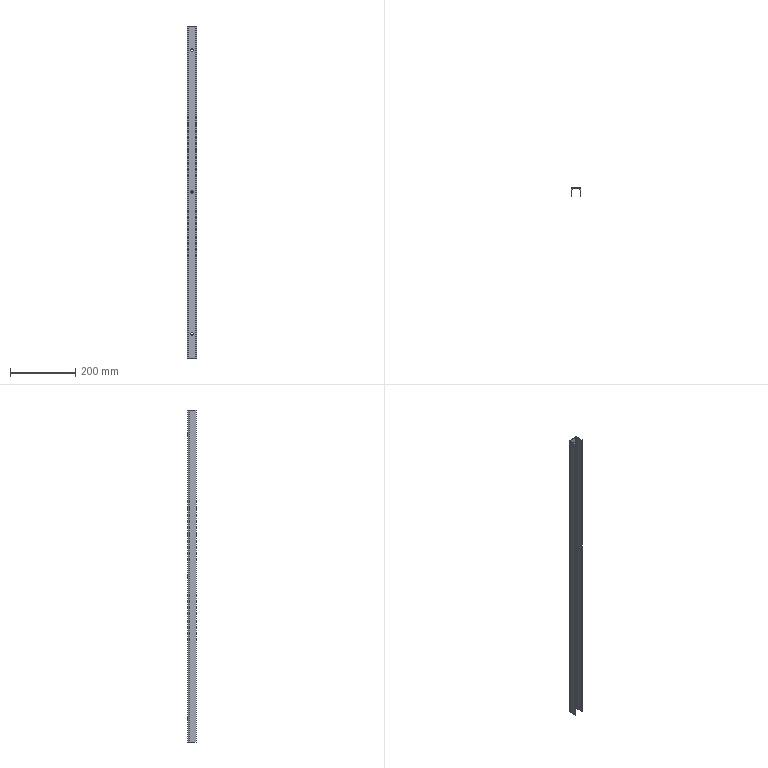Part | STEP file | SYL_0392D6J1SYL0380DJ10-1470572 | 1 solid | 28 faces | box 30 x 25 x 1018 mm | volume 149191 mm3 | plane 18 | cylinder 10 | commonest cylinder face diameters 8 x8 4 x2
STEP:
#1=CARTESIAN_POINT('',(0.,23.,-439.));
#2=VERTEX_POINT('',#1);
#3=CARTESIAN_POINT('',(0.,25.,-439.));
#4=VERTEX_POINT('',#3);
#5=CARTESIAN_POINT('',(0.,25.,-439.));
#6=DIRECTION('',(0.,1.,0.));
#7=VECTOR('',#6,1000.);
#8=LINE('',#5,#7);
#9=EDGE_CURVE('',#2,#4,#8,.T.);
#10=ORIENTED_EDGE('',*,*,#9,.F.);
#11=CARTESIAN_POINT('',(0.,23.,-431.));
#12=VERTEX_POINT('',#11);
#13=CARTESIAN_POINT('',(0.,23.,-435.));
#14=DIRECTION('',(0.,-1.,0.));
#15=DIRECTION('',(0.,0.,-1.));
#16=AXIS2_PLACEMENT_3D('',#13,#14,#15);
#17=CIRCLE('',#16,4.);
#18=EDGE_CURVE('',#2,#12,#17,.T.);
#19=ORIENTED_EDGE('',*,*,#18,.T.);
#20=CARTESIAN_POINT('',(0.,25.,-431.));
#21=VERTEX_POINT('',#20);
#22=CARTESIAN_POINT('',(0.,25.,-431.));
#23=DIRECTION('',(0.,1.,0.));
#24=VECTOR('',#23,1000.);
#25=LINE('',#22,#24);
#26=EDGE_CURVE('',#12,#21,#25,.T.);
#27=ORIENTED_EDGE('',*,*,#26,.T.);
#28=CARTESIAN_POINT('',(0.,25.,-435.));
#29=DIRECTION('',(0.,-1.,0.));
#30=DIRECTION('',(0.,0.,-1.));
#31=AXIS2_PLACEMENT_3D('',#28,#29,#30);
#32=CIRCLE('',#31,4.);
#33=EDGE_CURVE('',#4,#21,#32,.T.);
#34=ORIENTED_EDGE('',*,*,#33,.F.);
#35=EDGE_LOOP('',(#10,#19,#27,#34));
#36=FACE_OUTER_BOUND('',#35,.T.);
#37=CARTESIAN_POINT('',(0.,25.,-435.));
#38=DIRECTION('',(0.,1.,0.));
#39=DIRECTION('',(0.,0.,1.));
#40=AXIS2_PLACEMENT_3D('',#37,#38,#39);
#41=CYLINDRICAL_SURFACE('',#40,4.);
#42=ADVANCED_FACE('',(#36),#41,.F.);
#43=CARTESIAN_POINT('',(0.,23.,-4.));
#44=VERTEX_POINT('',#43);
#45=CARTESIAN_POINT('',(0.,25.,-4.));
#46=VERTEX_POINT('',#45);
#47=CARTESIAN_POINT('',(0.,25.,-4.));
#48=DIRECTION('',(0.,1.,0.));
#49=VECTOR('',#48,1000.);
#50=LINE('',#47,#49);
#51=EDGE_CURVE('',#44,#46,#50,.T.);
#52=ORIENTED_EDGE('',*,*,#51,.F.);
#53=CARTESIAN_POINT('',(0.,23.,4.));
#54=VERTEX_POINT('',#53);
#55=CARTESIAN_POINT('',(0.,23.,0.));
#56=DIRECTION('',(0.,-1.,0.));
#57=DIRECTION('',(0.,0.,-1.));
#58=AXIS2_PLACEMENT_3D('',#55,#56,#57);
#59=CIRCLE('',#58,4.);
#60=EDGE_CURVE('',#44,#54,#59,.T.);
#61=ORIENTED_EDGE('',*,*,#60,.T.);
#62=CARTESIAN_POINT('',(0.,25.,4.));
#63=VERTEX_POINT('',#62);
#64=CARTESIAN_POINT('',(0.,25.,4.));
#65=DIRECTION('',(0.,1.,0.));
#66=VECTOR('',#65,1000.);
#67=LINE('',#64,#66);
#68=EDGE_CURVE('',#54,#63,#67,.T.);
#69=ORIENTED_EDGE('',*,*,#68,.T.);
#70=CARTESIAN_POINT('',(0.,25.,0.));
#71=DIRECTION('',(0.,-1.,0.));
#72=DIRECTION('',(0.,0.,-1.));
#73=AXIS2_PLACEMENT_3D('',#70,#71,#72);
#74=CIRCLE('',#73,4.);
#75=EDGE_CURVE('',#46,#63,#74,.T.);
#76=ORIENTED_EDGE('',*,*,#75,.F.);
#77=EDGE_LOOP('',(#52,#61,#69,#76));
#78=FACE_OUTER_BOUND('',#77,.T.);
#79=CARTESIAN_POINT('',(0.,25.,0.));
#80=DIRECTION('',(0.,1.,0.));
#81=DIRECTION('',(0.,0.,1.));
#82=AXIS2_PLACEMENT_3D('',#79,#80,#81);
#83=CYLINDRICAL_SURFACE('',#82,4.);
#84=ADVANCED_FACE('',(#78),#83,.F.);
#85=CARTESIAN_POINT('',(0.,23.,431.));
#86=VERTEX_POINT('',#85);
#87=CARTESIAN_POINT('',(0.,25.,431.));
#88=VERTEX_POINT('',#87);
#89=CARTESIAN_POINT('',(0.,25.,431.));
#90=DIRECTION('',(0.,1.,0.));
#91=VECTOR('',#90,1000.);
#92=LINE('',#89,#91);
#93=EDGE_CURVE('',#86,#88,#92,.T.);
#94=ORIENTED_EDGE('',*,*,#93,.F.);
#95=CARTESIAN_POINT('',(0.,23.,439.));
#96=VERTEX_POINT('',#95);
#97=CARTESIAN_POINT('',(0.,23.,435.));
#98=DIRECTION('',(0.,-1.,0.));
#99=DIRECTION('',(0.,0.,-1.));
#100=AXIS2_PLACEMENT_3D('',#97,#98,#99);
#101=CIRCLE('',#100,4.);
#102=EDGE_CURVE('',#86,#96,#101,.T.);
#103=ORIENTED_EDGE('',*,*,#102,.T.);
#104=CARTESIAN_POINT('',(0.,25.,439.));
#105=VERTEX_POINT('',#104);
#106=CARTESIAN_POINT('',(0.,25.,439.));
#107=DIRECTION('',(0.,1.,0.));
#108=VECTOR('',#107,1000.);
#109=LINE('',#106,#108);
#110=EDGE_CURVE('',#96,#105,#109,.T.);
#111=ORIENTED_EDGE('',*,*,#110,.T.);
#112=CARTESIAN_POINT('',(0.,25.,435.));
#113=DIRECTION('',(0.,-1.,0.));
#114=DIRECTION('',(0.,0.,-1.));
#115=AXIS2_PLACEMENT_3D('',#112,#113,#114);
#116=CIRCLE('',#115,4.);
#117=EDGE_CURVE('',#88,#105,#116,.T.);
#118=ORIENTED_EDGE('',*,*,#117,.F.);
#119=EDGE_LOOP('',(#94,#103,#111,#118));
#120=FACE_OUTER_BOUND('',#119,.T.);
#121=CARTESIAN_POINT('',(0.,25.,435.));
#122=DIRECTION('',(0.,1.,0.));
#123=DIRECTION('',(0.,0.,1.));
#124=AXIS2_PLACEMENT_3D('',#121,#122,#123);
#125=CYLINDRICAL_SURFACE('',#124,4.);
#126=ADVANCED_FACE('',(#120),#125,.F.);
#127=CARTESIAN_POINT('',(-13.,0.,-509.));
#128=VERTEX_POINT('',#127);
#129=CARTESIAN_POINT('',(-15.,0.,-509.));
#130=VERTEX_POINT('',#129);
#131=CARTESIAN_POINT('',(-15.,0.,-509.));
#132=DIRECTION('',(-1.,0.,0.));
#133=VECTOR('',#132,1000.);
#134=LINE('',#131,#133);
#135=EDGE_CURVE('',#128,#130,#134,.T.);
#136=ORIENTED_EDGE('',*,*,#135,.F.);
#137=CARTESIAN_POINT('',(-13.,0.,509.));
#138=VERTEX_POINT('',#137);
#139=CARTESIAN_POINT('',(-13.,0.,-509.));
#140=DIRECTION('',(0.,0.,1.));
#141=VECTOR('',#140,1000.);
#142=LINE('',#139,#141);
#143=EDGE_CURVE('',#128,#138,#142,.T.);
#144=ORIENTED_EDGE('',*,*,#143,.T.);
#145=CARTESIAN_POINT('',(-15.,0.,509.));
#146=VERTEX_POINT('',#145);
#147=CARTESIAN_POINT('',(-15.,0.,509.));
#148=DIRECTION('',(-1.,0.,0.));
#149=VECTOR('',#148,1000.);
#150=LINE('',#147,#149);
#151=EDGE_CURVE('',#138,#146,#150,.T.);
#152=ORIENTED_EDGE('',*,*,#151,.T.);
#153=CARTESIAN_POINT('',(-15.,0.,-509.));
#154=DIRECTION('',(0.,0.,1.));
#155=VECTOR('',#154,1000.);
#156=LINE('',#153,#155);
#157=EDGE_CURVE('',#130,#146,#156,.T.);
#158=ORIENTED_EDGE('',*,*,#157,.F.);
#159=EDGE_LOOP('',(#136,#144,#152,#158));
#160=FACE_OUTER_BOUND('',#159,.T.);
#161=CARTESIAN_POINT('',(-15.,0.,-509.));
#162=DIRECTION('',(0.,-1.,0.));
#163=DIRECTION('',(0.,0.,1.));
#164=AXIS2_PLACEMENT_3D('',#161,#162,#163);
#165=PLANE('',#164);
#166=ADVANCED_FACE('',(#160),#165,.T.);
#167=ORIENTED_EDGE('',*,*,#151,.F.);
#168=CARTESIAN_POINT('',(-13.,21.,509.));
#169=VERTEX_POINT('',#168);
#170=CARTESIAN_POINT('',(-13.,21.,509.));
#171=DIRECTION('',(0.,-1.,0.));
#172=VECTOR('',#171,1000.);
#173=LINE('',#170,#172);
#174=EDGE_CURVE('',#169,#138,#173,.T.);
#175=ORIENTED_EDGE('',*,*,#174,.F.);
#176=CARTESIAN_POINT('',(-15.,21.,509.));
#177=VERTEX_POINT('',#176);
#178=CARTESIAN_POINT('',(-15.,21.,509.));
#179=DIRECTION('',(-1.,0.,0.));
#180=VECTOR('',#179,1000.);
#181=LINE('',#178,#180);
#182=EDGE_CURVE('',#169,#177,#181,.T.);
#183=ORIENTED_EDGE('',*,*,#182,.T.);
#184=CARTESIAN_POINT('',(-15.,21.,509.));
#185=DIRECTION('',(0.,-1.,0.));
#186=VECTOR('',#185,1000.);
#187=LINE('',#184,#186);
#188=EDGE_CURVE('',#177,#146,#187,.T.);
#189=ORIENTED_EDGE('',*,*,#188,.T.);
#190=EDGE_LOOP('',(#167,#175,#183,#189));
#191=FACE_OUTER_BOUND('',#190,.T.);
#192=CARTESIAN_POINT('',(-15.,21.,509.));
#193=DIRECTION('',(0.,0.,-1.));
#194=DIRECTION('',(0.,-1.,0.));
#195=AXIS2_PLACEMENT_3D('',#192,#193,#194);
#196=PLANE('',#195);
#197=ADVANCED_FACE('',(#191),#196,.F.);
#198=ORIENTED_EDGE('',*,*,#182,.F.);
#199=CARTESIAN_POINT('',(-11.,23.,509.));
#200=VERTEX_POINT('',#199);
#201=CARTESIAN_POINT('',(-11.,21.,509.));
#202=DIRECTION('',(0.,0.,1.));
#203=DIRECTION('',(1.,0.,0.));
#204=AXIS2_PLACEMENT_3D('',#201,#202,#203);
#205=CIRCLE('',#204,2.);
#206=EDGE_CURVE('',#200,#169,#205,.T.);
#207=ORIENTED_EDGE('',*,*,#206,.F.);
#208=CARTESIAN_POINT('',(-11.,25.,509.));
#209=VERTEX_POINT('',#208);
#210=CARTESIAN_POINT('',(-11.,25.,509.));
#211=DIRECTION('',(0.,1.,0.));
#212=VECTOR('',#211,1000.);
#213=LINE('',#210,#212);
#214=EDGE_CURVE('',#200,#209,#213,.T.);
#215=ORIENTED_EDGE('',*,*,#214,.T.);
#216=CARTESIAN_POINT('',(-11.,21.,509.));
#217=DIRECTION('',(0.,0.,1.));
#218=DIRECTION('',(0.,1.,0.));
#219=AXIS2_PLACEMENT_3D('',#216,#217,#218);
#220=CIRCLE('',#219,4.);
#221=EDGE_CURVE('',#209,#177,#220,.T.);
#222=ORIENTED_EDGE('',*,*,#221,.T.);
#223=EDGE_LOOP('',(#198,#207,#215,#222));
#224=FACE_OUTER_BOUND('',#223,.T.);
#225=CARTESIAN_POINT('',(-11.,21.,509.));
#226=DIRECTION('',(0.,0.,-1.));
#227=DIRECTION('',(-1.,0.,0.));
#228=AXIS2_PLACEMENT_3D('',#225,#226,#227);
#229=PLANE('',#228);
#230=ADVANCED_FACE('',(#224),#229,.F.);
#231=ORIENTED_EDGE('',*,*,#214,.F.);
#232=CARTESIAN_POINT('',(11.,23.,509.));
#233=VERTEX_POINT('',#232);
#234=CARTESIAN_POINT('',(11.,23.,509.));
#235=DIRECTION('',(-1.,0.,0.));
#236=VECTOR('',#235,1000.);
#237=LINE('',#234,#236);
#238=EDGE_CURVE('',#233,#200,#237,.T.);
#239=ORIENTED_EDGE('',*,*,#238,.F.);
#240=CARTESIAN_POINT('',(11.,25.,509.));
#241=VERTEX_POINT('',#240);
#242=CARTESIAN_POINT('',(11.,25.,509.));
#243=DIRECTION('',(0.,1.,0.));
#244=VECTOR('',#243,1000.);
#245=LINE('',#242,#244);
#246=EDGE_CURVE('',#233,#241,#245,.T.);
#247=ORIENTED_EDGE('',*,*,#246,.T.);
#248=CARTESIAN_POINT('',(11.,25.,509.));
#249=DIRECTION('',(-1.,0.,0.));
#250=VECTOR('',#249,1000.);
#251=LINE('',#248,#250);
#252=EDGE_CURVE('',#241,#209,#251,.T.);
#253=ORIENTED_EDGE('',*,*,#252,.T.);
#254=EDGE_LOOP('',(#231,#239,#247,#253));
#255=FACE_OUTER_BOUND('',#254,.T.);
#256=CARTESIAN_POINT('',(11.,25.,509.));
#257=DIRECTION('',(0.,0.,-1.));
#258=DIRECTION('',(-1.,0.,0.));
#259=AXIS2_PLACEMENT_3D('',#256,#257,#258);
#260=PLANE('',#259);
#261=ADVANCED_FACE('',(#255),#260,.F.);
#262=ORIENTED_EDGE('',*,*,#246,.F.);
#263=CARTESIAN_POINT('',(13.,21.,509.));
#264=VERTEX_POINT('',#263);
#265=CARTESIAN_POINT('',(11.,21.,509.));
#266=DIRECTION('',(0.,0.,1.));
#267=DIRECTION('',(1.,0.,0.));
#268=AXIS2_PLACEMENT_3D('',#265,#266,#267);
#269=CIRCLE('',#268,2.);
#270=EDGE_CURVE('',#264,#233,#269,.T.);
#271=ORIENTED_EDGE('',*,*,#270,.F.);
#272=CARTESIAN_POINT('',(15.,21.,509.));
#273=VERTEX_POINT('',#272);
#274=CARTESIAN_POINT('',(15.,21.,509.));
#275=DIRECTION('',(1.,0.,0.));
#276=VECTOR('',#275,1000.);
#277=LINE('',#274,#276);
#278=EDGE_CURVE('',#264,#273,#277,.T.);
#279=ORIENTED_EDGE('',*,*,#278,.T.);
#280=CARTESIAN_POINT('',(11.,21.,509.));
#281=DIRECTION('',(0.,0.,1.));
#282=DIRECTION('',(1.,0.,0.));
#283=AXIS2_PLACEMENT_3D('',#280,#281,#282);
#284=CIRCLE('',#283,4.);
#285=EDGE_CURVE('',#273,#241,#284,.T.);
#286=ORIENTED_EDGE('',*,*,#285,.T.);
#287=EDGE_LOOP('',(#262,#271,#279,#286));
#288=FACE_OUTER_BOUND('',#287,.T.);
#289=CARTESIAN_POINT('',(11.,21.,509.));
#290=DIRECTION('',(0.,0.,-1.));
#291=DIRECTION('',(-1.,0.,0.));
#292=AXIS2_PLACEMENT_3D('',#289,#290,#291);
#293=PLANE('',#292);
#294=ADVANCED_FACE('',(#288),#293,.F.);
#295=ORIENTED_EDGE('',*,*,#278,.F.);
#296=CARTESIAN_POINT('',(13.,0.,509.));
#297=VERTEX_POINT('',#296);
#298=CARTESIAN_POINT('',(13.,0.,509.));
#299=DIRECTION('',(0.,1.,0.));
#300=VECTOR('',#299,1000.);
#301=LINE('',#298,#300);
#302=EDGE_CURVE('',#297,#264,#301,.T.);
#303=ORIENTED_EDGE('',*,*,#302,.F.);
#304=CARTESIAN_POINT('',(15.,0.,509.));
#305=VERTEX_POINT('',#304);
#306=CARTESIAN_POINT('',(15.,0.,509.));
#307=DIRECTION('',(1.,0.,0.));
#308=VECTOR('',#307,1000.);
#309=LINE('',#306,#308);
#310=EDGE_CURVE('',#297,#305,#309,.T.);
#311=ORIENTED_EDGE('',*,*,#310,.T.);
#312=CARTESIAN_POINT('',(15.,0.,509.));
#313=DIRECTION('',(0.,1.,0.));
#314=VECTOR('',#313,1000.);
#315=LINE('',#312,#314);
#316=EDGE_CURVE('',#305,#273,#315,.T.);
#317=ORIENTED_EDGE('',*,*,#316,.T.);
#318=EDGE_LOOP('',(#295,#303,#311,#317));
#319=FACE_OUTER_BOUND('',#318,.T.);
#320=CARTESIAN_POINT('',(15.,0.,509.));
#321=DIRECTION('',(0.,0.,-1.));
#322=DIRECTION('',(0.,1.,0.));
#323=AXIS2_PLACEMENT_3D('',#320,#321,#322);
#324=PLANE('',#323);
#325=ADVANCED_FACE('',(#319),#324,.F.);
#326=ORIENTED_EDGE('',*,*,#310,.F.);
#327=CARTESIAN_POINT('',(13.,0.,-509.));
#328=VERTEX_POINT('',#327);
#329=CARTESIAN_POINT('',(13.,0.,-509.));
#330=DIRECTION('',(0.,0.,1.));
#331=VECTOR('',#330,1000.);
#332=LINE('',#329,#331);
#333=EDGE_CURVE('',#328,#297,#332,.T.);
#334=ORIENTED_EDGE('',*,*,#333,.F.);
#335=CARTESIAN_POINT('',(15.,0.,-509.));
#336=VERTEX_POINT('',#335);
#337=CARTESIAN_POINT('',(15.,0.,-509.));
#338=DIRECTION('',(1.,0.,0.));
#339=VECTOR('',#338,1000.);
#340=LINE('',#337,#339);
#341=EDGE_CURVE('',#328,#336,#340,.T.);
#342=ORIENTED_EDGE('',*,*,#341,.T.);
#343=CARTESIAN_POINT('',(15.,0.,-509.));
#344=DIRECTION('',(0.,0.,1.));
#345=VECTOR('',#344,1000.);
#346=LINE('',#343,#345);
#347=EDGE_CURVE('',#336,#305,#346,.T.);
#348=ORIENTED_EDGE('',*,*,#347,.T.);
#349=EDGE_LOOP('',(#326,#334,#342,#348));
#350=FACE_OUTER_BOUND('',#349,.T.);
#351=CARTESIAN_POINT('',(15.,0.,-509.));
#352=DIRECTION('',(0.,1.,0.));
#353=DIRECTION('',(0.,0.,1.));
#354=AXIS2_PLACEMENT_3D('',#351,#352,#353);
#355=PLANE('',#354);
#356=ADVANCED_FACE('',(#350),#355,.F.);
#357=ORIENTED_EDGE('',*,*,#341,.F.);
#358=CARTESIAN_POINT('',(13.,21.,-509.));
#359=VERTEX_POINT('',#358);
#360=CARTESIAN_POINT('',(13.,0.,-509.));
#361=DIRECTION('',(0.,1.,0.));
#362=VECTOR('',#361,1000.);
#363=LINE('',#360,#362);
#364=EDGE_CURVE('',#328,#359,#363,.T.);
#365=ORIENTED_EDGE('',*,*,#364,.T.);
#366=CARTESIAN_POINT('',(15.,21.,-509.));
#367=VERTEX_POINT('',#366);
#368=CARTESIAN_POINT('',(15.,21.,-509.));
#369=DIRECTION('',(1.,0.,0.));
#370=VECTOR('',#369,1000.);
#371=LINE('',#368,#370);
#372=EDGE_CURVE('',#359,#367,#371,.T.);
#373=ORIENTED_EDGE('',*,*,#372,.T.);
#374=CARTESIAN_POINT('',(15.,0.,-509.));
#375=DIRECTION('',(0.,1.,0.));
#376=VECTOR('',#375,1000.);
#377=LINE('',#374,#376);
#378=EDGE_CURVE('',#336,#367,#377,.T.);
#379=ORIENTED_EDGE('',*,*,#378,.F.);
#380=EDGE_LOOP('',(#357,#365,#373,#379));
#381=FACE_OUTER_BOUND('',#380,.T.);
#382=CARTESIAN_POINT('',(15.,0.,-509.));
#383=DIRECTION('',(0.,0.,-1.));
#384=DIRECTION('',(0.,1.,0.));
#385=AXIS2_PLACEMENT_3D('',#382,#383,#384);
#386=PLANE('',#385);
#387=ADVANCED_FACE('',(#381),#386,.T.);
#388=ORIENTED_EDGE('',*,*,#372,.F.);
#389=CARTESIAN_POINT('',(11.,23.,-509.));
#390=VERTEX_POINT('',#389);
#391=CARTESIAN_POINT('',(11.,21.,-509.));
#392=DIRECTION('',(0.,0.,-1.));
#393=DIRECTION('',(1.,0.,0.));
#394=AXIS2_PLACEMENT_3D('',#391,#392,#393);
#395=CIRCLE('',#394,2.);
#396=EDGE_CURVE('',#390,#359,#395,.T.);
#397=ORIENTED_EDGE('',*,*,#396,.F.);
#398=CARTESIAN_POINT('',(11.,25.,-509.));
#399=VERTEX_POINT('',#398);
#400=CARTESIAN_POINT('',(11.,25.,-509.));
#401=DIRECTION('',(0.,1.,0.));
#402=VECTOR('',#401,1000.);
#403=LINE('',#400,#402);
#404=EDGE_CURVE('',#390,#399,#403,.T.);
#405=ORIENTED_EDGE('',*,*,#404,.T.);
#406=CARTESIAN_POINT('',(11.,21.,-509.));
#407=DIRECTION('',(0.,0.,-1.));
#408=DIRECTION('',(0.,1.,0.));
#409=AXIS2_PLACEMENT_3D('',#406,#407,#408);
#410=CIRCLE('',#409,4.);
#411=EDGE_CURVE('',#399,#367,#410,.T.);
#412=ORIENTED_EDGE('',*,*,#411,.T.);
#413=EDGE_LOOP('',(#388,#397,#405,#412));
#414=FACE_OUTER_BOUND('',#413,.T.);
#415=CARTESIAN_POINT('',(11.,21.,-509.));
#416=DIRECTION('',(0.,0.,1.));
#417=DIRECTION('',(1.,0.,0.));
#418=AXIS2_PLACEMENT_3D('',#415,#416,#417);
#419=PLANE('',#418);
#420=ADVANCED_FACE('',(#414),#419,.F.);
#421=ORIENTED_EDGE('',*,*,#404,.F.);
#422=CARTESIAN_POINT('',(-11.,23.,-509.));
#423=VERTEX_POINT('',#422);
#424=CARTESIAN_POINT('',(11.,23.,-509.));
#425=DIRECTION('',(-1.,0.,0.));
#426=VECTOR('',#425,1000.);
#427=LINE('',#424,#426);
#428=EDGE_CURVE('',#390,#423,#427,.T.);
#429=ORIENTED_EDGE('',*,*,#428,.T.);
#430=CARTESIAN_POINT('',(-11.,25.,-509.));
#431=VERTEX_POINT('',#430);
#432=CARTESIAN_POINT('',(-11.,25.,-509.));
#433=DIRECTION('',(0.,1.,0.));
#434=VECTOR('',#433,1000.);
#435=LINE('',#432,#434);
#436=EDGE_CURVE('',#423,#431,#435,.T.);
#437=ORIENTED_EDGE('',*,*,#436,.T.);
#438=CARTESIAN_POINT('',(11.,25.,-509.));
#439=DIRECTION('',(-1.,0.,0.));
#440=VECTOR('',#439,1000.);
#441=LINE('',#438,#440);
#442=EDGE_CURVE('',#399,#431,#441,.T.);
#443=ORIENTED_EDGE('',*,*,#442,.F.);
#444=EDGE_LOOP('',(#421,#429,#437,#443));
#445=FACE_OUTER_BOUND('',#444,.T.);
#446=CARTESIAN_POINT('',(11.,25.,-509.));
#447=DIRECTION('',(0.,0.,-1.));
#448=DIRECTION('',(-1.,0.,0.));
#449=AXIS2_PLACEMENT_3D('',#446,#447,#448);
#450=PLANE('',#449);
#451=ADVANCED_FACE('',(#445),#450,.T.);
#452=ORIENTED_EDGE('',*,*,#436,.F.);
#453=CARTESIAN_POINT('',(-13.,21.,-509.));
#454=VERTEX_POINT('',#453);
#455=CARTESIAN_POINT('',(-11.,21.,-509.));
#456=DIRECTION('',(0.,0.,-1.));
#457=DIRECTION('',(1.,0.,0.));
#458=AXIS2_PLACEMENT_3D('',#455,#456,#457);
#459=CIRCLE('',#458,2.);
#460=EDGE_CURVE('',#454,#423,#459,.T.);
#461=ORIENTED_EDGE('',*,*,#460,.F.);
#462=CARTESIAN_POINT('',(-15.,21.,-509.));
#463=VERTEX_POINT('',#462);
#464=CARTESIAN_POINT('',(-15.,21.,-509.));
#465=DIRECTION('',(-1.,0.,0.));
#466=VECTOR('',#465,1000.);
#467=LINE('',#464,#466);
#468=EDGE_CURVE('',#454,#463,#467,.T.);
#469=ORIENTED_EDGE('',*,*,#468,.T.);
#470=CARTESIAN_POINT('',(-11.,21.,-509.));
#471=DIRECTION('',(0.,0.,-1.));
#472=DIRECTION('',(-1.,0.,0.));
#473=AXIS2_PLACEMENT_3D('',#470,#471,#472);
#474=CIRCLE('',#473,4.);
#475=EDGE_CURVE('',#463,#431,#474,.T.);
#476=ORIENTED_EDGE('',*,*,#475,.T.);
#477=EDGE_LOOP('',(#452,#461,#469,#476));
#478=FACE_OUTER_BOUND('',#477,.T.);
#479=CARTESIAN_POINT('',(-11.,21.,-509.));
#480=DIRECTION('',(0.,0.,1.));
#481=DIRECTION('',(1.,0.,0.));
#482=AXIS2_PLACEMENT_3D('',#479,#480,#481);
#483=PLANE('',#482);
#484=ADVANCED_FACE('',(#478),#483,.F.);
#485=CARTESIAN_POINT('',(0.,23.,435.));
#486=DIRECTION('',(0.,-1.,0.));
#487=DIRECTION('',(0.,0.,-1.));
#488=AXIS2_PLACEMENT_3D('',#485,#486,#487);
#489=CIRCLE('',#488,4.);
#490=EDGE_CURVE('',#96,#86,#489,.T.);
#491=ORIENTED_EDGE('',*,*,#490,.T.);
#492=ORIENTED_EDGE('',*,*,#93,.T.);
#493=CARTESIAN_POINT('',(0.,25.,435.));
#494=DIRECTION('',(0.,-1.,0.));
#495=DIRECTION('',(0.,0.,1.));
#496=AXIS2_PLACEMENT_3D('',#493,#494,#495);
#497=CIRCLE('',#496,4.);
#498=EDGE_CURVE('',#105,#88,#497,.T.);
#499=ORIENTED_EDGE('',*,*,#498,.F.);
#500=ORIENTED_EDGE('',*,*,#110,.F.);
#501=EDGE_LOOP('',(#491,#492,#499,#500));
#502=FACE_OUTER_BOUND('',#501,.T.);
#503=CARTESIAN_POINT('',(0.,25.,435.));
#504=DIRECTION('',(0.,1.,0.));
#505=DIRECTION('',(0.,0.,1.));
#506=AXIS2_PLACEMENT_3D('',#503,#504,#505);
#507=CYLINDRICAL_SURFACE('',#506,4.);
#508=ADVANCED_FACE('',(#502),#507,.F.);
#509=CARTESIAN_POINT('',(0.,23.,0.));
#510=DIRECTION('',(0.,-1.,0.));
#511=DIRECTION('',(0.,0.,-1.));
#512=AXIS2_PLACEMENT_3D('',#509,#510,#511);
#513=CIRCLE('',#512,4.);
#514=EDGE_CURVE('',#54,#44,#513,.T.);
#515=ORIENTED_EDGE('',*,*,#514,.T.);
#516=ORIENTED_EDGE('',*,*,#51,.T.);
#517=CARTESIAN_POINT('',(0.,25.,0.));
#518=DIRECTION('',(0.,-1.,0.));
#519=DIRECTION('',(0.,0.,1.));
#520=AXIS2_PLACEMENT_3D('',#517,#518,#519);
#521=CIRCLE('',#520,4.);
#522=EDGE_CURVE('',#63,#46,#521,.T.);
#523=ORIENTED_EDGE('',*,*,#522,.F.);
#524=ORIENTED_EDGE('',*,*,#68,.F.);
#525=EDGE_LOOP('',(#515,#516,#523,#524));
#526=FACE_OUTER_BOUND('',#525,.T.);
#527=CARTESIAN_POINT('',(0.,25.,0.));
#528=DIRECTION('',(0.,1.,0.));
#529=DIRECTION('',(0.,0.,1.));
#530=AXIS2_PLACEMENT_3D('',#527,#528,#529);
#531=CYLINDRICAL_SURFACE('',#530,4.);
#532=ADVANCED_FACE('',(#526),#531,.F.);
#533=CARTESIAN_POINT('',(0.,23.,-435.));
#534=DIRECTION('',(0.,-1.,0.));
#535=DIRECTION('',(0.,0.,-1.));
#536=AXIS2_PLACEMENT_3D('',#533,#534,#535);
#537=CIRCLE('',#536,4.);
#538=EDGE_CURVE('',#12,#2,#537,.T.);
#539=ORIENTED_EDGE('',*,*,#538,.T.);
#540=ORIENTED_EDGE('',*,*,#9,.T.);
#541=CARTESIAN_POINT('',(0.,25.,-435.));
#542=DIRECTION('',(0.,-1.,0.));
#543=DIRECTION('',(0.,0.,1.));
#544=AXIS2_PLACEMENT_3D('',#541,#542,#543);
#545=CIRCLE('',#544,4.);
#546=EDGE_CURVE('',#21,#4,#545,.T.);
#547=ORIENTED_EDGE('',*,*,#546,.F.);
#548=ORIENTED_EDGE('',*,*,#26,.F.);
#549=EDGE_LOOP('',(#539,#540,#547,#548));
#550=FACE_OUTER_BOUND('',#549,.T.);
#551=CARTESIAN_POINT('',(0.,25.,-435.));
#552=DIRECTION('',(0.,1.,0.));
#553=DIRECTION('',(0.,0.,1.));
#554=AXIS2_PLACEMENT_3D('',#551,#552,#553);
#555=CYLINDRICAL_SURFACE('',#554,4.);
#556=ADVANCED_FACE('',(#550),#555,.F.);
#557=CARTESIAN_POINT('',(-13.,21.,-509.));
#558=DIRECTION('',(0.,-1.,0.));
#559=VECTOR('',#558,1000.);
#560=LINE('',#557,#559);
#561=EDGE_CURVE('',#454,#128,#560,.T.);
#562=ORIENTED_EDGE('',*,*,#561,.T.);
#563=ORIENTED_EDGE('',*,*,#135,.T.);
#564=CARTESIAN_POINT('',(-15.,21.,-509.));
#565=DIRECTION('',(0.,-1.,0.));
#566=VECTOR('',#565,1000.);
#567=LINE('',#564,#566);
#568=EDGE_CURVE('',#463,#130,#567,.T.);
#569=ORIENTED_EDGE('',*,*,#568,.F.);
#570=ORIENTED_EDGE('',*,*,#468,.F.);
#571=EDGE_LOOP('',(#562,#563,#569,#570));
#572=FACE_OUTER_BOUND('',#571,.T.);
#573=CARTESIAN_POINT('',(-15.,21.,-509.));
#574=DIRECTION('',(0.,0.,-1.));
#575=DIRECTION('',(0.,-1.,0.));
#576=AXIS2_PLACEMENT_3D('',#573,#574,#575);
#577=PLANE('',#576);
#578=ADVANCED_FACE('',(#572),#577,.T.);
#579=ORIENTED_EDGE('',*,*,#475,.F.);
#580=CARTESIAN_POINT('',(-15.,21.,-509.));
#581=DIRECTION('',(0.,0.,1.));
#582=VECTOR('',#581,1000.);
#583=LINE('',#580,#582);
#584=EDGE_CURVE('',#463,#177,#583,.T.);
#585=ORIENTED_EDGE('',*,*,#584,.T.);
#586=ORIENTED_EDGE('',*,*,#221,.F.);
#587=CARTESIAN_POINT('',(-11.,25.,509.));
#588=DIRECTION('',(0.,0.,-1.));
#589=VECTOR('',#588,1000.);
#590=LINE('',#587,#589);
#591=EDGE_CURVE('',#209,#431,#590,.T.);
#592=ORIENTED_EDGE('',*,*,#591,.T.);
#593=EDGE_LOOP('',(#579,#585,#586,#592));
#594=FACE_OUTER_BOUND('',#593,.T.);
#595=CARTESIAN_POINT('',(-11.,21.,-509.));
#596=DIRECTION('',(0.,0.,1.));
#597=DIRECTION('',(1.,0.,0.));
#598=AXIS2_PLACEMENT_3D('',#595,#596,#597);
#599=CYLINDRICAL_SURFACE('',#598,4.);
#600=ADVANCED_FACE('',(#594),#599,.T.);
#601=ORIENTED_EDGE('',*,*,#568,.T.);
#602=ORIENTED_EDGE('',*,*,#157,.T.);
#603=ORIENTED_EDGE('',*,*,#188,.F.);
#604=ORIENTED_EDGE('',*,*,#584,.F.);
#605=EDGE_LOOP('',(#601,#602,#603,#604));
#606=FACE_OUTER_BOUND('',#605,.T.);
#607=CARTESIAN_POINT('',(-15.,21.,-509.));
#608=DIRECTION('',(-1.,0.,0.));
#609=DIRECTION('',(0.,0.,1.));
#610=AXIS2_PLACEMENT_3D('',#607,#608,#609);
#611=PLANE('',#610);
#612=ADVANCED_FACE('',(#606),#611,.T.);
#613=ORIENTED_EDGE('',*,*,#411,.F.);
#614=CARTESIAN_POINT('',(11.,25.,-509.));
#615=DIRECTION('',(0.,0.,1.));
#616=VECTOR('',#615,1000.);
#617=LINE('',#614,#616);
#618=EDGE_CURVE('',#399,#241,#617,.T.);
#619=ORIENTED_EDGE('',*,*,#618,.T.);
#620=ORIENTED_EDGE('',*,*,#285,.F.);
#621=CARTESIAN_POINT('',(15.,21.,509.));
#622=DIRECTION('',(0.,0.,-1.));
#623=VECTOR('',#622,1000.);
#624=LINE('',#621,#623);
#625=EDGE_CURVE('',#273,#367,#624,.T.);
#626=ORIENTED_EDGE('',*,*,#625,.T.);
#627=EDGE_LOOP('',(#613,#619,#620,#626));
#628=FACE_OUTER_BOUND('',#627,.T.);
#629=CARTESIAN_POINT('',(11.,21.,-509.));
#630=DIRECTION('',(0.,0.,1.));
#631=DIRECTION('',(1.,0.,0.));
#632=AXIS2_PLACEMENT_3D('',#629,#630,#631);
#633=CYLINDRICAL_SURFACE('',#632,4.);
#634=ADVANCED_FACE('',(#628),#633,.T.);
#635=ORIENTED_EDGE('',*,*,#378,.T.);
#636=ORIENTED_EDGE('',*,*,#625,.F.);
#637=ORIENTED_EDGE('',*,*,#316,.F.);
#638=ORIENTED_EDGE('',*,*,#347,.F.);
#639=EDGE_LOOP('',(#635,#636,#637,#638));
#640=FACE_OUTER_BOUND('',#639,.T.);
#641=CARTESIAN_POINT('',(15.,0.,-509.));
#642=DIRECTION('',(1.,0.,0.));
#643=DIRECTION('',(0.,1.,0.));
#644=AXIS2_PLACEMENT_3D('',#641,#642,#643);
#645=PLANE('',#644);
#646=ADVANCED_FACE('',(#640),#645,.T.);
#647=ORIENTED_EDGE('',*,*,#117,.T.);
#648=ORIENTED_EDGE('',*,*,#498,.T.);
#649=EDGE_LOOP('',(#647,#648));
#650=FACE_BOUND('',#649,.T.);
#651=ORIENTED_EDGE('',*,*,#75,.T.);
#652=ORIENTED_EDGE('',*,*,#522,.T.);
#653=EDGE_LOOP('',(#651,#652));
#654=FACE_BOUND('',#653,.T.);
#655=ORIENTED_EDGE('',*,*,#33,.T.);
#656=ORIENTED_EDGE('',*,*,#546,.T.);
#657=EDGE_LOOP('',(#655,#656));
#658=FACE_BOUND('',#657,.T.);
#659=ORIENTED_EDGE('',*,*,#442,.T.);
#660=ORIENTED_EDGE('',*,*,#591,.F.);
#661=ORIENTED_EDGE('',*,*,#252,.F.);
#662=ORIENTED_EDGE('',*,*,#618,.F.);
#663=EDGE_LOOP('',(#659,#660,#661,#662));
#664=FACE_OUTER_BOUND('',#663,.T.);
#665=CARTESIAN_POINT('',(11.,25.,-509.));
#666=DIRECTION('',(0.,1.,0.));
#667=DIRECTION('',(1.,0.,0.));
#668=AXIS2_PLACEMENT_3D('',#665,#666,#667);
#669=PLANE('',#668);
#670=ADVANCED_FACE('',(#650,#654,#658,#664),#669,.T.);
#671=ORIENTED_EDGE('',*,*,#460,.T.);
#672=CARTESIAN_POINT('',(-11.,23.,-509.));
#673=DIRECTION('',(0.,0.,-1.));
#674=VECTOR('',#673,1000.);
#675=LINE('',#672,#674);
#676=EDGE_CURVE('',#200,#423,#675,.T.);
#677=ORIENTED_EDGE('',*,*,#676,.F.);
#678=ORIENTED_EDGE('',*,*,#206,.T.);
#679=CARTESIAN_POINT('',(-13.,21.,-509.));
#680=DIRECTION('',(0.,0.,1.));
#681=VECTOR('',#680,1000.);
#682=LINE('',#679,#681);
#683=EDGE_CURVE('',#454,#169,#682,.T.);
#684=ORIENTED_EDGE('',*,*,#683,.F.);
#685=EDGE_LOOP('',(#671,#677,#678,#684));
#686=FACE_OUTER_BOUND('',#685,.T.);
#687=CARTESIAN_POINT('',(-11.,21.,-509.));
#688=DIRECTION('',(0.,0.,1.));
#689=DIRECTION('',(1.,0.,0.));
#690=AXIS2_PLACEMENT_3D('',#687,#688,#689);
#691=CYLINDRICAL_SURFACE('',#690,2.);
#692=ADVANCED_FACE('',(#686),#691,.F.);
#693=ORIENTED_EDGE('',*,*,#561,.F.);
#694=ORIENTED_EDGE('',*,*,#683,.T.);
#695=ORIENTED_EDGE('',*,*,#174,.T.);
#696=ORIENTED_EDGE('',*,*,#143,.F.);
#697=EDGE_LOOP('',(#693,#694,#695,#696));
#698=FACE_OUTER_BOUND('',#697,.T.);
#699=CARTESIAN_POINT('',(-13.,21.,-509.));
#700=DIRECTION('',(-1.,0.,0.));
#701=DIRECTION('',(0.,0.,1.));
#702=AXIS2_PLACEMENT_3D('',#699,#700,#701);
#703=PLANE('',#702);
#704=ADVANCED_FACE('',(#698),#703,.F.);
#705=ORIENTED_EDGE('',*,*,#396,.T.);
#706=CARTESIAN_POINT('',(13.,21.,-509.));
#707=DIRECTION('',(0.,0.,-1.));
#708=VECTOR('',#707,1000.);
#709=LINE('',#706,#708);
#710=EDGE_CURVE('',#264,#359,#709,.T.);
#711=ORIENTED_EDGE('',*,*,#710,.F.);
#712=ORIENTED_EDGE('',*,*,#270,.T.);
#713=CARTESIAN_POINT('',(11.,23.,-509.));
#714=DIRECTION('',(0.,0.,1.));
#715=VECTOR('',#714,1000.);
#716=LINE('',#713,#715);
#717=EDGE_CURVE('',#390,#233,#716,.T.);
#718=ORIENTED_EDGE('',*,*,#717,.F.);
#719=EDGE_LOOP('',(#705,#711,#712,#718));
#720=FACE_OUTER_BOUND('',#719,.T.);
#721=CARTESIAN_POINT('',(11.,21.,-509.));
#722=DIRECTION('',(0.,0.,1.));
#723=DIRECTION('',(1.,0.,0.));
#724=AXIS2_PLACEMENT_3D('',#721,#722,#723);
#725=CYLINDRICAL_SURFACE('',#724,2.);
#726=ADVANCED_FACE('',(#720),#725,.F.);
#727=ORIENTED_EDGE('',*,*,#364,.F.);
#728=ORIENTED_EDGE('',*,*,#333,.T.);
#729=ORIENTED_EDGE('',*,*,#302,.T.);
#730=ORIENTED_EDGE('',*,*,#710,.T.);
#731=EDGE_LOOP('',(#727,#728,#729,#730));
#732=FACE_OUTER_BOUND('',#731,.T.);
#733=CARTESIAN_POINT('',(13.,0.,-509.));
#734=DIRECTION('',(1.,0.,0.));
#735=DIRECTION('',(0.,1.,0.));
#736=AXIS2_PLACEMENT_3D('',#733,#734,#735);
#737=PLANE('',#736);
#738=ADVANCED_FACE('',(#732),#737,.F.);
#739=ORIENTED_EDGE('',*,*,#102,.F.);
#740=ORIENTED_EDGE('',*,*,#490,.F.);
#741=EDGE_LOOP('',(#739,#740));
#742=FACE_BOUND('',#741,.T.);
#743=ORIENTED_EDGE('',*,*,#60,.F.);
#744=ORIENTED_EDGE('',*,*,#514,.F.);
#745=EDGE_LOOP('',(#743,#744));
#746=FACE_BOUND('',#745,.T.);
#747=ORIENTED_EDGE('',*,*,#18,.F.);
#748=ORIENTED_EDGE('',*,*,#538,.F.);
#749=EDGE_LOOP('',(#747,#748));
#750=FACE_BOUND('',#749,.T.);
#751=ORIENTED_EDGE('',*,*,#428,.F.);
#752=ORIENTED_EDGE('',*,*,#717,.T.);
#753=ORIENTED_EDGE('',*,*,#238,.T.);
#754=ORIENTED_EDGE('',*,*,#676,.T.);
#755=EDGE_LOOP('',(#751,#752,#753,#754));
#756=FACE_OUTER_BOUND('',#755,.T.);
#757=CARTESIAN_POINT('',(11.,23.,-509.));
#758=DIRECTION('',(0.,1.,0.));
#759=DIRECTION('',(1.,0.,0.));
#760=AXIS2_PLACEMENT_3D('',#757,#758,#759);
#761=PLANE('',#760);
#762=ADVANCED_FACE('',(#742,#746,#750,#756),#761,.F.);
#763=CLOSED_SHELL('',(#42,#84,#126,#166,#197,#230,#261,#294,#325,#356,#387,#420,#451,#484,#508,#532,#556,#578,#600,#612,#634,#646,#670,#692,#704,#726,#738,#762));
#764=MANIFOLD_SOLID_BREP('',#763);
#765=CARTESIAN_POINT('',(0.,0.,0.));
#766=DIRECTION('',(0.,0.,1.));
#767=DIRECTION('',(1.,0.,0.));
#768=AXIS2_PLACEMENT_3D('',#765,#766,#767);
#769=(LENGTH_UNIT()NAMED_UNIT(*)SI_UNIT(.MILLI.,.METRE.));
#770=UNCERTAINTY_MEASURE_WITH_UNIT(LENGTH_MEASURE(0.00001),#769,'','');
#771=(NAMED_UNIT(*)PLANE_ANGLE_UNIT()SI_UNIT($,.RADIAN.));
#772=(NAMED_UNIT(*)SI_UNIT($,.STERADIAN.)SOLID_ANGLE_UNIT());
#773=(GEOMETRIC_REPRESENTATION_CONTEXT(3)GLOBAL_UNCERTAINTY_ASSIGNED_CONTEXT((#770))GLOBAL_UNIT_ASSIGNED_CONTEXT((#769,#771,#772))REPRESENTATION_CONTEXT('',''));
#774=ADVANCED_BREP_SHAPE_REPRESENTATION('',(#764,#768),#773);